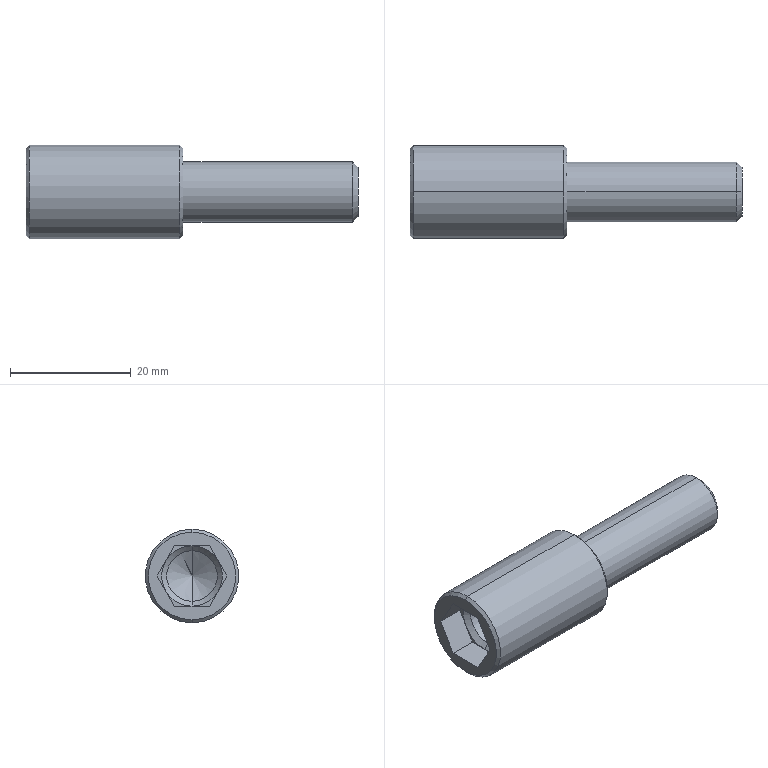Part | STEP file | SI100_25 | 1 solid | 31 faces | box 55 x 15.5 x 15.5 mm | volume 5807 mm3 | plane 15 | cone 10 | cylinder 6 | commonest cylinder face diameters 8.376 x2 10 x2 15.5 x2